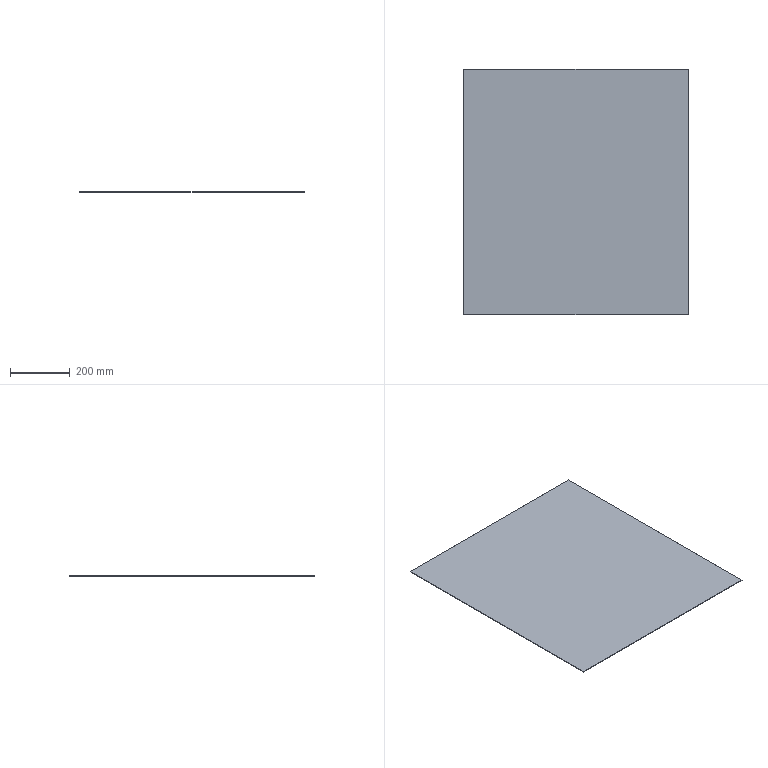Part | STEP file | Part 3 PN_0001_ASM 2 | 1 solid | 6 faces | box 751.5 x 821.5 x 2 mm | volume 1234714 mm3 | plane 6
STEP:
#1=CARTESIAN_POINT('',(20.,860.,0.));
#2=VERTEX_POINT('',#1);
#3=CARTESIAN_POINT('',(20.,38.5,0.));
#4=VERTEX_POINT('',#3);
#5=CARTESIAN_POINT('',(20.,860.,0.));
#6=DIRECTION('',(0.,-1.,0.));
#7=VECTOR('',#6,1000.);
#8=LINE('',#5,#7);
#9=EDGE_CURVE('',#2,#4,#8,.T.);
#10=ORIENTED_EDGE('',*,*,#9,.F.);
#11=CARTESIAN_POINT('',(20.,860.,-2.));
#12=VERTEX_POINT('',#11);
#13=CARTESIAN_POINT('',(20.,860.,-2.));
#14=DIRECTION('',(0.,0.,1.));
#15=VECTOR('',#14,1000.);
#16=LINE('',#13,#15);
#17=EDGE_CURVE('',#12,#2,#16,.T.);
#18=ORIENTED_EDGE('',*,*,#17,.F.);
#19=CARTESIAN_POINT('',(20.,38.5,-2.));
#20=VERTEX_POINT('',#19);
#21=CARTESIAN_POINT('',(20.,860.,-2.));
#22=DIRECTION('',(0.,-1.,0.));
#23=VECTOR('',#22,1000.);
#24=LINE('',#21,#23);
#25=EDGE_CURVE('',#12,#20,#24,.T.);
#26=ORIENTED_EDGE('',*,*,#25,.T.);
#27=CARTESIAN_POINT('',(20.,38.5,-2.));
#28=DIRECTION('',(0.,0.,1.));
#29=VECTOR('',#28,1000.);
#30=LINE('',#27,#29);
#31=EDGE_CURVE('',#20,#4,#30,.T.);
#32=ORIENTED_EDGE('',*,*,#31,.T.);
#33=EDGE_LOOP('',(#10,#18,#26,#32));
#34=FACE_OUTER_BOUND('',#33,.T.);
#35=CARTESIAN_POINT('',(20.,860.,-2.));
#36=DIRECTION('',(-1.,0.,0.));
#37=DIRECTION('',(0.,0.,1.));
#38=AXIS2_PLACEMENT_3D('',#35,#36,#37);
#39=PLANE('',#38);
#40=ADVANCED_FACE('',(#34),#39,.T.);
#41=CARTESIAN_POINT('',(771.5,860.,0.));
#42=VERTEX_POINT('',#41);
#43=CARTESIAN_POINT('',(20.,860.,0.));
#44=DIRECTION('',(-1.,0.,0.));
#45=VECTOR('',#44,1000.);
#46=LINE('',#43,#45);
#47=EDGE_CURVE('',#42,#2,#46,.T.);
#48=ORIENTED_EDGE('',*,*,#47,.F.);
#49=CARTESIAN_POINT('',(771.5,860.,-2.));
#50=VERTEX_POINT('',#49);
#51=CARTESIAN_POINT('',(771.5,860.,-2.));
#52=DIRECTION('',(0.,0.,1.));
#53=VECTOR('',#52,1000.);
#54=LINE('',#51,#53);
#55=EDGE_CURVE('',#50,#42,#54,.T.);
#56=ORIENTED_EDGE('',*,*,#55,.F.);
#57=CARTESIAN_POINT('',(20.,860.,-2.));
#58=DIRECTION('',(-1.,0.,0.));
#59=VECTOR('',#58,1000.);
#60=LINE('',#57,#59);
#61=EDGE_CURVE('',#50,#12,#60,.T.);
#62=ORIENTED_EDGE('',*,*,#61,.T.);
#63=ORIENTED_EDGE('',*,*,#17,.T.);
#64=EDGE_LOOP('',(#48,#56,#62,#63));
#65=FACE_OUTER_BOUND('',#64,.T.);
#66=CARTESIAN_POINT('',(20.,860.,-2.));
#67=DIRECTION('',(0.,1.,0.));
#68=DIRECTION('',(0.,0.,1.));
#69=AXIS2_PLACEMENT_3D('',#66,#67,#68);
#70=PLANE('',#69);
#71=ADVANCED_FACE('',(#65),#70,.T.);
#72=CARTESIAN_POINT('',(771.5,38.5,0.));
#73=VERTEX_POINT('',#72);
#74=CARTESIAN_POINT('',(771.5,860.,0.));
#75=DIRECTION('',(0.,1.,0.));
#76=VECTOR('',#75,1000.);
#77=LINE('',#74,#76);
#78=EDGE_CURVE('',#73,#42,#77,.T.);
#79=ORIENTED_EDGE('',*,*,#78,.F.);
#80=CARTESIAN_POINT('',(771.5,38.5,-2.));
#81=VERTEX_POINT('',#80);
#82=CARTESIAN_POINT('',(771.5,38.5,-2.));
#83=DIRECTION('',(0.,0.,1.));
#84=VECTOR('',#83,1000.);
#85=LINE('',#82,#84);
#86=EDGE_CURVE('',#81,#73,#85,.T.);
#87=ORIENTED_EDGE('',*,*,#86,.F.);
#88=CARTESIAN_POINT('',(771.5,860.,-2.));
#89=DIRECTION('',(0.,1.,0.));
#90=VECTOR('',#89,1000.);
#91=LINE('',#88,#90);
#92=EDGE_CURVE('',#81,#50,#91,.T.);
#93=ORIENTED_EDGE('',*,*,#92,.T.);
#94=ORIENTED_EDGE('',*,*,#55,.T.);
#95=EDGE_LOOP('',(#79,#87,#93,#94));
#96=FACE_OUTER_BOUND('',#95,.T.);
#97=CARTESIAN_POINT('',(771.5,860.,-2.));
#98=DIRECTION('',(1.,0.,0.));
#99=DIRECTION('',(0.,1.,0.));
#100=AXIS2_PLACEMENT_3D('',#97,#98,#99);
#101=PLANE('',#100);
#102=ADVANCED_FACE('',(#96),#101,.T.);
#103=CARTESIAN_POINT('',(20.,38.5,0.));
#104=DIRECTION('',(1.,0.,0.));
#105=VECTOR('',#104,1000.);
#106=LINE('',#103,#105);
#107=EDGE_CURVE('',#4,#73,#106,.T.);
#108=ORIENTED_EDGE('',*,*,#107,.F.);
#109=ORIENTED_EDGE('',*,*,#31,.F.);
#110=CARTESIAN_POINT('',(20.,38.5,-2.));
#111=DIRECTION('',(1.,0.,0.));
#112=VECTOR('',#111,1000.);
#113=LINE('',#110,#112);
#114=EDGE_CURVE('',#20,#81,#113,.T.);
#115=ORIENTED_EDGE('',*,*,#114,.T.);
#116=ORIENTED_EDGE('',*,*,#86,.T.);
#117=EDGE_LOOP('',(#108,#109,#115,#116));
#118=FACE_OUTER_BOUND('',#117,.T.);
#119=CARTESIAN_POINT('',(20.,38.5,-2.));
#120=DIRECTION('',(0.,-1.,0.));
#121=DIRECTION('',(0.,0.,-1.));
#122=AXIS2_PLACEMENT_3D('',#119,#120,#121);
#123=PLANE('',#122);
#124=ADVANCED_FACE('',(#118),#123,.T.);
#125=ORIENTED_EDGE('',*,*,#25,.F.);
#126=ORIENTED_EDGE('',*,*,#61,.F.);
#127=ORIENTED_EDGE('',*,*,#92,.F.);
#128=ORIENTED_EDGE('',*,*,#114,.F.);
#129=EDGE_LOOP('',(#125,#126,#127,#128));
#130=FACE_OUTER_BOUND('',#129,.T.);
#131=CARTESIAN_POINT('',(20.,38.5,-2.));
#132=DIRECTION('',(0.,0.,1.));
#133=DIRECTION('',(1.,0.,0.));
#134=AXIS2_PLACEMENT_3D('',#131,#132,#133);
#135=PLANE('',#134);
#136=ADVANCED_FACE('',(#130),#135,.F.);
#137=ORIENTED_EDGE('',*,*,#9,.T.);
#138=ORIENTED_EDGE('',*,*,#107,.T.);
#139=ORIENTED_EDGE('',*,*,#78,.T.);
#140=ORIENTED_EDGE('',*,*,#47,.T.);
#141=EDGE_LOOP('',(#137,#138,#139,#140));
#142=FACE_OUTER_BOUND('',#141,.T.);
#143=CARTESIAN_POINT('',(20.,38.5,0.));
#144=DIRECTION('',(0.,0.,1.));
#145=DIRECTION('',(1.,0.,0.));
#146=AXIS2_PLACEMENT_3D('',#143,#144,#145);
#147=PLANE('',#146);
#148=ADVANCED_FACE('',(#142),#147,.T.);
#149=CLOSED_SHELL('',(#40,#71,#102,#124,#136,#148));
#150=MANIFOLD_SOLID_BREP('',#149);
#151=CARTESIAN_POINT('',(0.,0.,0.));
#152=DIRECTION('',(0.,0.,1.));
#153=DIRECTION('',(1.,0.,0.));
#154=AXIS2_PLACEMENT_3D('',#151,#152,#153);
#155=(LENGTH_UNIT()NAMED_UNIT(*)SI_UNIT(.MILLI.,.METRE.));
#156=UNCERTAINTY_MEASURE_WITH_UNIT(LENGTH_MEASURE(0.00001),#155,'','');
#157=(NAMED_UNIT(*)PLANE_ANGLE_UNIT()SI_UNIT($,.RADIAN.));
#158=(NAMED_UNIT(*)SI_UNIT($,.STERADIAN.)SOLID_ANGLE_UNIT());
#159=(GEOMETRIC_REPRESENTATION_CONTEXT(3)GLOBAL_UNCERTAINTY_ASSIGNED_CONTEXT((#156))GLOBAL_UNIT_ASSIGNED_CONTEXT((#155,#157,#158))REPRESENTATION_CONTEXT('',''));
#160=ADVANCED_BREP_SHAPE_REPRESENTATION('',(#150,#154),#159);